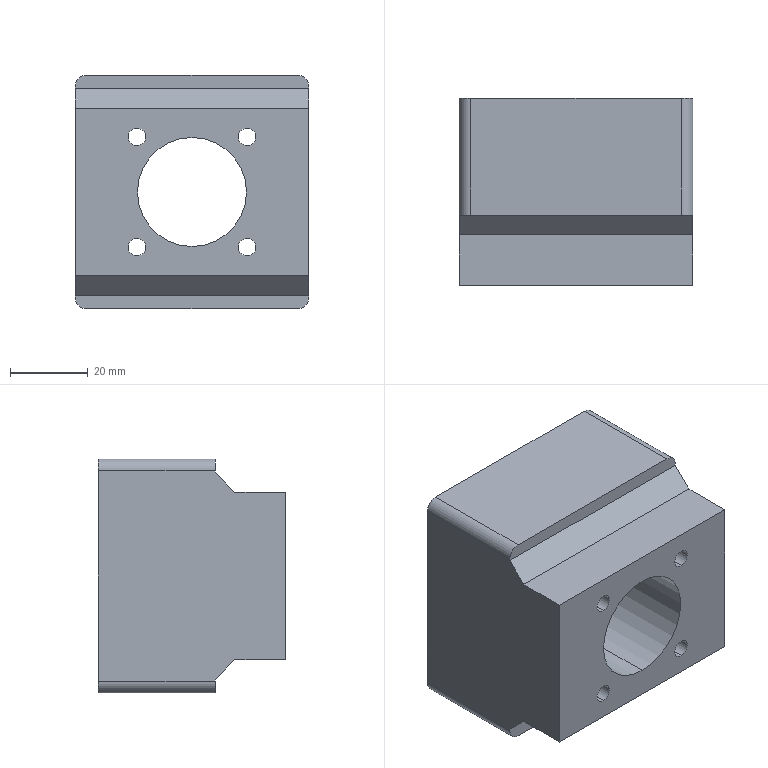Part | STEP file | 10-24 reducer mounting seat | 1 solid | 57 faces | box 60 x 48 x 60 mm | volume 97911 mm3 | cylinder 32 | plane 17 | cone 8 | commonest cylinder face diameters 4.2 x8 4.5 x8 10.59 x8 6 x4 28 x2 56 x2